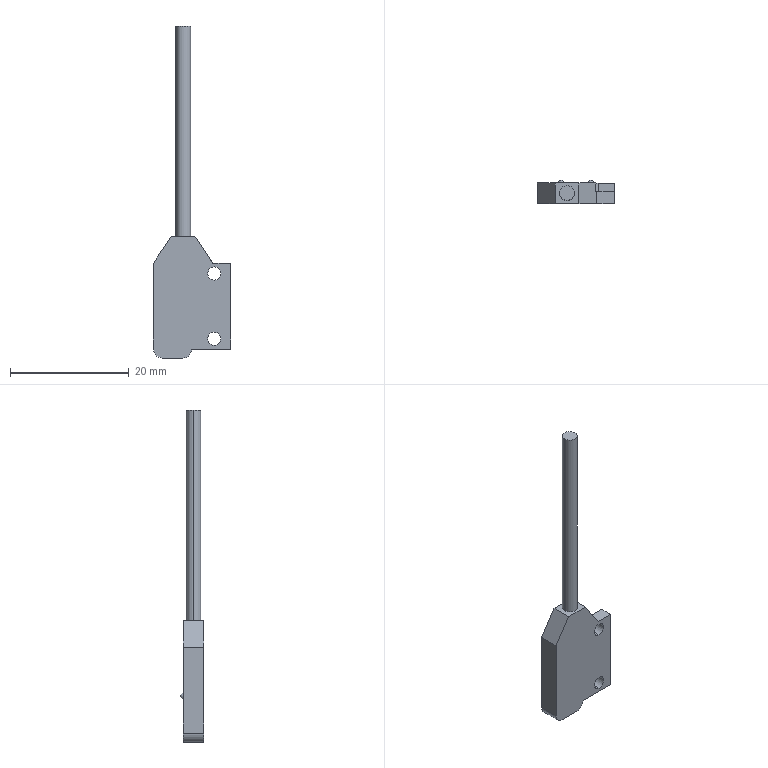Part | SolidWorks | features ICE 4, Chamfer 2, Fillet 2, Extrusion 1 | 1 solid | 28 faces | box 13 x 4 x 56 mm | volume 912.44 mm3 | plane 16 | cylinder 10 | sphere 2 | commonest cylinder face diameters 2.2 x4 2.5 x2 3 x2 4 x2
STEP:
#1=CARTESIAN_POINT('',(-0.25,1.75,47.25));
#2=VERTEX_POINT('',#1);
#3=CARTESIAN_POINT('',(-2.75,1.75,47.25));
#4=VERTEX_POINT('',#3);
#5=CARTESIAN_POINT('',(-1.5,1.75,47.25));
#6=DIRECTION('',(0.,0.,1.));
#7=DIRECTION('',(1.,0.,0.));
#8=AXIS2_PLACEMENT_3D('',#5,#6,#7);
#9=CIRCLE('',#8,1.25);
#10=EDGE_CURVE('',#2,#4,#9,.T.);
#11=ORIENTED_EDGE('',*,*,#10,.F.);
#12=CARTESIAN_POINT('',(-0.25,1.75,11.75));
#13=VERTEX_POINT('',#12);
#14=CARTESIAN_POINT('',(-0.25,1.75,47.25));
#15=DIRECTION('',(0.,0.,-1.));
#16=VECTOR('',#15,1000.);
#17=LINE('',#14,#16);
#18=EDGE_CURVE('',#2,#13,#17,.T.);
#19=ORIENTED_EDGE('',*,*,#18,.T.);
#20=CARTESIAN_POINT('',(-2.75,1.75,11.75));
#21=VERTEX_POINT('',#20);
#22=CARTESIAN_POINT('',(-1.5,1.75,11.75));
#23=DIRECTION('',(0.,0.,1.));
#24=DIRECTION('',(-1.,0.,0.));
#25=AXIS2_PLACEMENT_3D('',#22,#23,#24);
#26=CIRCLE('',#25,1.25);
#27=EDGE_CURVE('',#13,#21,#26,.T.);
#28=ORIENTED_EDGE('',*,*,#27,.T.);
#29=CARTESIAN_POINT('',(-2.75,1.75,47.25));
#30=DIRECTION('',(0.,0.,-1.));
#31=VECTOR('',#30,1000.);
#32=LINE('',#29,#31);
#33=EDGE_CURVE('',#4,#21,#32,.T.);
#34=ORIENTED_EDGE('',*,*,#33,.F.);
#35=EDGE_LOOP('',(#11,#19,#28,#34));
#36=FACE_OUTER_BOUND('',#35,.T.);
#37=CARTESIAN_POINT('',(-1.5,1.75,47.25));
#38=DIRECTION('',(0.,0.,-1.));
#39=DIRECTION('',(-1.,0.,0.));
#40=AXIS2_PLACEMENT_3D('',#37,#38,#39);
#41=CYLINDRICAL_SURFACE('',#40,1.25);
#42=ADVANCED_FACE('',(#36),#41,.T.);
#43=CARTESIAN_POINT('',(3.75,0.,-6.6));
#44=VERTEX_POINT('',#43);
#45=CARTESIAN_POINT('',(3.75,0.,-4.4));
#46=VERTEX_POINT('',#45);
#47=CARTESIAN_POINT('',(3.75,0.,-5.5));
#48=DIRECTION('',(0.,1.,0.));
#49=DIRECTION('',(0.,0.,1.));
#50=AXIS2_PLACEMENT_3D('',#47,#48,#49);
#51=CIRCLE('',#50,1.1);
#52=EDGE_CURVE('',#44,#46,#51,.T.);
#53=ORIENTED_EDGE('',*,*,#52,.F.);
#54=CARTESIAN_POINT('',(3.75,2.1,-6.6));
#55=VERTEX_POINT('',#54);
#56=CARTESIAN_POINT('',(3.75,-1.5,-6.6));
#57=DIRECTION('',(0.,1.,0.));
#58=VECTOR('',#57,1000.);
#59=LINE('',#56,#58);
#60=EDGE_CURVE('',#44,#55,#59,.T.);
#61=ORIENTED_EDGE('',*,*,#60,.T.);
#62=CARTESIAN_POINT('',(3.75,2.1,-4.4));
#63=VERTEX_POINT('',#62);
#64=CARTESIAN_POINT('',(3.75,2.1,-5.5));
#65=DIRECTION('',(0.,-1.,0.));
#66=DIRECTION('',(0.,0.,1.));
#67=AXIS2_PLACEMENT_3D('',#64,#65,#66);
#68=CIRCLE('',#67,1.1);
#69=EDGE_CURVE('',#63,#55,#68,.T.);
#70=ORIENTED_EDGE('',*,*,#69,.F.);
#71=CARTESIAN_POINT('',(3.75,-1.5,-4.4));
#72=DIRECTION('',(0.,1.,0.));
#73=VECTOR('',#72,1000.);
#74=LINE('',#71,#73);
#75=EDGE_CURVE('',#46,#63,#74,.T.);
#76=ORIENTED_EDGE('',*,*,#75,.F.);
#77=EDGE_LOOP('',(#53,#61,#70,#76));
#78=FACE_OUTER_BOUND('',#77,.T.);
#79=CARTESIAN_POINT('',(3.75,-1.5,-5.5));
#80=DIRECTION('',(0.,1.,0.));
#81=DIRECTION('',(0.,0.,1.));
#82=AXIS2_PLACEMENT_3D('',#79,#80,#81);
#83=CYLINDRICAL_SURFACE('',#82,1.1);
#84=ADVANCED_FACE('',(#78),#83,.F.);
#85=CARTESIAN_POINT('',(3.75,0.,4.4));
#86=VERTEX_POINT('',#85);
#87=CARTESIAN_POINT('',(3.75,0.,6.6));
#88=VERTEX_POINT('',#87);
#89=CARTESIAN_POINT('',(3.75,0.,5.5));
#90=DIRECTION('',(0.,1.,0.));
#91=DIRECTION('',(0.,0.,1.));
#92=AXIS2_PLACEMENT_3D('',#89,#90,#91);
#93=CIRCLE('',#92,1.1);
#94=EDGE_CURVE('',#86,#88,#93,.T.);
#95=ORIENTED_EDGE('',*,*,#94,.F.);
#96=CARTESIAN_POINT('',(3.75,2.1,4.4));
#97=VERTEX_POINT('',#96);
#98=CARTESIAN_POINT('',(3.75,-1.5,4.4));
#99=DIRECTION('',(0.,1.,0.));
#100=VECTOR('',#99,1000.);
#101=LINE('',#98,#100);
#102=EDGE_CURVE('',#86,#97,#101,.T.);
#103=ORIENTED_EDGE('',*,*,#102,.T.);
#104=CARTESIAN_POINT('',(3.75,2.1,6.6));
#105=VERTEX_POINT('',#104);
#106=CARTESIAN_POINT('',(3.75,2.1,5.5));
#107=DIRECTION('',(0.,-1.,0.));
#108=DIRECTION('',(0.,0.,1.));
#109=AXIS2_PLACEMENT_3D('',#106,#107,#108);
#110=CIRCLE('',#109,1.1);
#111=EDGE_CURVE('',#105,#97,#110,.T.);
#112=ORIENTED_EDGE('',*,*,#111,.F.);
#113=CARTESIAN_POINT('',(3.75,-1.5,6.6));
#114=DIRECTION('',(0.,1.,0.));
#115=VECTOR('',#114,1000.);
#116=LINE('',#113,#115);
#117=EDGE_CURVE('',#88,#105,#116,.T.);
#118=ORIENTED_EDGE('',*,*,#117,.F.);
#119=EDGE_LOOP('',(#95,#103,#112,#118));
#120=FACE_OUTER_BOUND('',#119,.T.);
#121=CARTESIAN_POINT('',(3.75,-1.5,5.5));
#122=DIRECTION('',(0.,1.,0.));
#123=DIRECTION('',(0.,0.,1.));
#124=AXIS2_PLACEMENT_3D('',#121,#122,#123);
#125=CYLINDRICAL_SURFACE('',#124,1.1);
#126=ADVANCED_FACE('',(#120),#125,.F.);
#127=CARTESIAN_POINT('',(3.5,2.1,7.25));
#128=VERTEX_POINT('',#127);
#129=CARTESIAN_POINT('',(6.5,2.1,7.25));
#130=VERTEX_POINT('',#129);
#131=CARTESIAN_POINT('',(3.5,2.1,7.25));
#132=DIRECTION('',(1.,0.,0.));
#133=VECTOR('',#132,1000.);
#134=LINE('',#131,#133);
#135=EDGE_CURVE('',#128,#130,#134,.T.);
#136=ORIENTED_EDGE('',*,*,#135,.F.);
#137=CARTESIAN_POINT('',(3.5,0.,7.25));
#138=VERTEX_POINT('',#137);
#139=CARTESIAN_POINT('',(3.5,3.5,7.25));
#140=DIRECTION('',(0.,-1.,0.));
#141=VECTOR('',#140,1000.);
#142=LINE('',#139,#141);
#143=EDGE_CURVE('',#128,#138,#142,.T.);
#144=ORIENTED_EDGE('',*,*,#143,.T.);
#145=CARTESIAN_POINT('',(6.5,0.,7.25));
#146=VERTEX_POINT('',#145);
#147=CARTESIAN_POINT('',(3.5,0.,7.25));
#148=DIRECTION('',(1.,0.,0.));
#149=VECTOR('',#148,1000.);
#150=LINE('',#147,#149);
#151=EDGE_CURVE('',#138,#146,#150,.T.);
#152=ORIENTED_EDGE('',*,*,#151,.T.);
#153=CARTESIAN_POINT('',(6.5,3.5,7.25));
#154=DIRECTION('',(0.,-1.,0.));
#155=VECTOR('',#154,1000.);
#156=LINE('',#153,#155);
#157=EDGE_CURVE('',#130,#146,#156,.T.);
#158=ORIENTED_EDGE('',*,*,#157,.F.);
#159=EDGE_LOOP('',(#136,#144,#152,#158));
#160=FACE_OUTER_BOUND('',#159,.T.);
#161=CARTESIAN_POINT('',(3.5,3.5,7.25));
#162=DIRECTION('',(0.,0.,-1.));
#163=DIRECTION('',(-1.,0.,0.));
#164=AXIS2_PLACEMENT_3D('',#161,#162,#163);
#165=PLANE('',#164);
#166=ADVANCED_FACE('',(#160),#165,.F.);
#167=ORIENTED_EDGE('',*,*,#102,.F.);
#168=CARTESIAN_POINT('',(3.75,0.,5.5));
#169=DIRECTION('',(0.,1.,0.));
#170=DIRECTION('',(0.,0.,1.));
#171=AXIS2_PLACEMENT_3D('',#168,#169,#170);
#172=CIRCLE('',#171,1.1);
#173=EDGE_CURVE('',#88,#86,#172,.T.);
#174=ORIENTED_EDGE('',*,*,#173,.F.);
#175=ORIENTED_EDGE('',*,*,#117,.T.);
#176=CARTESIAN_POINT('',(3.75,2.1,5.5));
#177=DIRECTION('',(0.,-1.,0.));
#178=DIRECTION('',(0.,0.,1.));
#179=AXIS2_PLACEMENT_3D('',#176,#177,#178);
#180=CIRCLE('',#179,1.1);
#181=EDGE_CURVE('',#97,#105,#180,.T.);
#182=ORIENTED_EDGE('',*,*,#181,.F.);
#183=EDGE_LOOP('',(#167,#174,#175,#182));
#184=FACE_OUTER_BOUND('',#183,.T.);
#185=CARTESIAN_POINT('',(3.75,-1.5,5.5));
#186=DIRECTION('',(0.,1.,0.));
#187=DIRECTION('',(0.,0.,1.));
#188=AXIS2_PLACEMENT_3D('',#185,#186,#187);
#189=CYLINDRICAL_SURFACE('',#188,1.1);
#190=ADVANCED_FACE('',(#184),#189,.F.);
#191=ORIENTED_EDGE('',*,*,#60,.F.);
#192=CARTESIAN_POINT('',(3.75,0.,-5.5));
#193=DIRECTION('',(0.,1.,0.));
#194=DIRECTION('',(0.,0.,1.));
#195=AXIS2_PLACEMENT_3D('',#192,#193,#194);
#196=CIRCLE('',#195,1.1);
#197=EDGE_CURVE('',#46,#44,#196,.T.);
#198=ORIENTED_EDGE('',*,*,#197,.F.);
#199=ORIENTED_EDGE('',*,*,#75,.T.);
#200=CARTESIAN_POINT('',(3.75,2.1,-5.5));
#201=DIRECTION('',(0.,-1.,0.));
#202=DIRECTION('',(0.,0.,1.));
#203=AXIS2_PLACEMENT_3D('',#200,#201,#202);
#204=CIRCLE('',#203,1.1);
#205=EDGE_CURVE('',#55,#63,#204,.T.);
#206=ORIENTED_EDGE('',*,*,#205,.F.);
#207=EDGE_LOOP('',(#191,#198,#199,#206));
#208=FACE_OUTER_BOUND('',#207,.T.);
#209=CARTESIAN_POINT('',(3.75,-1.5,-5.5));
#210=DIRECTION('',(0.,1.,0.));
#211=DIRECTION('',(0.,0.,1.));
#212=AXIS2_PLACEMENT_3D('',#209,#210,#211);
#213=CYLINDRICAL_SURFACE('',#212,1.1);
#214=ADVANCED_FACE('',(#208),#213,.F.);
#215=CARTESIAN_POINT('',(3.75,3.5,3.5));
#216=VERTEX_POINT('',#215);
#217=CARTESIAN_POINT('',(3.359,3.5,7.461));
#218=VERTEX_POINT('',#217);
#219=CARTESIAN_POINT('',(3.75,3.5,5.5));
#220=DIRECTION('',(0.,1.,0.));
#221=DIRECTION('',(0.,0.,1.));
#222=AXIS2_PLACEMENT_3D('',#219,#220,#221);
#223=CIRCLE('',#222,2.);
#224=EDGE_CURVE('',#216,#218,#223,.T.);
#225=ORIENTED_EDGE('',*,*,#224,.F.);
#226=CARTESIAN_POINT('',(6.5,3.5,3.5));
#227=VERTEX_POINT('',#226);
#228=CARTESIAN_POINT('',(3.75,3.5,3.5));
#229=DIRECTION('',(-1.,0.,0.));
#230=VECTOR('',#229,1000.);
#231=LINE('',#228,#230);
#232=EDGE_CURVE('',#227,#216,#231,.T.);
#233=ORIENTED_EDGE('',*,*,#232,.F.);
#234=CARTESIAN_POINT('',(6.5,3.5,-3.5));
#235=VERTEX_POINT('',#234);
#236=CARTESIAN_POINT('',(6.5,3.5,-7.25));
#237=DIRECTION('',(0.,0.,-1.));
#238=VECTOR('',#237,1000.);
#239=LINE('',#236,#238);
#240=EDGE_CURVE('',#227,#235,#239,.T.);
#241=ORIENTED_EDGE('',*,*,#240,.T.);
#242=CARTESIAN_POINT('',(3.75,3.5,-3.5));
#243=VERTEX_POINT('',#242);
#244=CARTESIAN_POINT('',(3.75,3.5,-3.5));
#245=DIRECTION('',(1.,0.,0.));
#246=VECTOR('',#245,1000.);
#247=LINE('',#244,#246);
#248=EDGE_CURVE('',#243,#235,#247,.T.);
#249=ORIENTED_EDGE('',*,*,#248,.F.);
#250=CARTESIAN_POINT('',(1.75,3.5,-5.5));
#251=VERTEX_POINT('',#250);
#252=CARTESIAN_POINT('',(3.75,3.5,-5.5));
#253=DIRECTION('',(0.,1.,0.));
#254=DIRECTION('',(0.,0.,1.));
#255=AXIS2_PLACEMENT_3D('',#252,#253,#254);
#256=CIRCLE('',#255,2.);
#257=EDGE_CURVE('',#251,#243,#256,.T.);
#258=ORIENTED_EDGE('',*,*,#257,.F.);
#259=CARTESIAN_POINT('',(1.75,3.5,-7.25));
#260=VERTEX_POINT('',#259);
#261=CARTESIAN_POINT('',(1.75,3.5,-7.25));
#262=DIRECTION('',(0.,0.,1.));
#263=VECTOR('',#262,1000.);
#264=LINE('',#261,#263);
#265=EDGE_CURVE('',#260,#251,#264,.T.);
#266=ORIENTED_EDGE('',*,*,#265,.F.);
#267=CARTESIAN_POINT('',(-0.05,3.5,-7.25));
#268=VERTEX_POINT('',#267);
#269=CARTESIAN_POINT('',(-0.05,3.5,-7.25));
#270=DIRECTION('',(-1.,0.,0.));
#271=VECTOR('',#270,1000.);
#272=LINE('',#269,#271);
#273=EDGE_CURVE('',#260,#268,#272,.T.);
#274=ORIENTED_EDGE('',*,*,#273,.T.);
#275=CARTESIAN_POINT('',(-1.55,3.5,-8.75));
#276=VERTEX_POINT('',#275);
#277=CARTESIAN_POINT('',(-1.55,3.5,-7.25));
#278=DIRECTION('',(0.,1.,0.));
#279=DIRECTION('',(0.,0.,1.));
#280=AXIS2_PLACEMENT_3D('',#277,#278,#279);
#281=CIRCLE('',#280,1.5);
#282=EDGE_CURVE('',#268,#276,#281,.T.);
#283=ORIENTED_EDGE('',*,*,#282,.T.);
#284=CARTESIAN_POINT('',(-5.,3.5,-8.75));
#285=VERTEX_POINT('',#284);
#286=CARTESIAN_POINT('',(-6.5,3.5,-8.75));
#287=DIRECTION('',(-1.,0.,0.));
#288=VECTOR('',#287,1000.);
#289=LINE('',#286,#288);
#290=EDGE_CURVE('',#276,#285,#289,.T.);
#291=ORIENTED_EDGE('',*,*,#290,.T.);
#292=CARTESIAN_POINT('',(-6.5,3.5,-7.25));
#293=VERTEX_POINT('',#292);
#294=CARTESIAN_POINT('',(-5.,3.5,-7.25));
#295=DIRECTION('',(0.,1.,0.));
#296=DIRECTION('',(0.,0.,1.));
#297=AXIS2_PLACEMENT_3D('',#294,#295,#296);
#298=CIRCLE('',#297,1.5);
#299=EDGE_CURVE('',#285,#293,#298,.T.);
#300=ORIENTED_EDGE('',*,*,#299,.T.);
#301=CARTESIAN_POINT('',(-6.5,3.5,7.25));
#302=VERTEX_POINT('',#301);
#303=CARTESIAN_POINT('',(-6.5,3.5,-8.75));
#304=DIRECTION('',(0.,0.,1.));
#305=VECTOR('',#304,1000.);
#306=LINE('',#303,#305);
#307=EDGE_CURVE('',#293,#302,#306,.T.);
#308=ORIENTED_EDGE('',*,*,#307,.T.);
#309=CARTESIAN_POINT('',(-3.5,3.5,11.75));
#310=VERTEX_POINT('',#309);
#311=CARTESIAN_POINT('',(-7.846,3.5,5.231));
#312=DIRECTION('',(0.5547,0.,0.8321));
#313=VECTOR('',#312,1000.);
#314=LINE('',#311,#313);
#315=EDGE_CURVE('',#302,#310,#314,.T.);
#316=ORIENTED_EDGE('',*,*,#315,.T.);
#317=CARTESIAN_POINT('',(0.5,3.5,11.75));
#318=VERTEX_POINT('',#317);
#319=CARTESIAN_POINT('',(-6.5,3.5,11.75));
#320=DIRECTION('',(1.,0.,0.));
#321=VECTOR('',#320,1000.);
#322=LINE('',#319,#321);
#323=EDGE_CURVE('',#310,#318,#322,.T.);
#324=ORIENTED_EDGE('',*,*,#323,.T.);
#325=CARTESIAN_POINT('',(5.769,3.5,3.846));
#326=DIRECTION('',(0.5547,0.,-0.8321));
#327=VECTOR('',#326,1000.);
#328=LINE('',#325,#327);
#329=EDGE_CURVE('',#318,#218,#328,.T.);
#330=ORIENTED_EDGE('',*,*,#329,.T.);
#331=EDGE_LOOP('',(#225,#233,#241,#249,#258,#266,#274,#283,#291,#300,#308,#316,#324,#330));
#332=FACE_OUTER_BOUND('',#331,.T.);
#333=CARTESIAN_POINT('',(-2.5,3.5,-0.5));
#334=VERTEX_POINT('',#333);
#335=CARTESIAN_POINT('',(-2.5,3.5,-1.5));
#336=VERTEX_POINT('',#335);
#337=CARTESIAN_POINT('',(-2.5,3.5,-1.));
#338=DIRECTION('',(0.,1.,0.));
#339=DIRECTION('',(0.,0.,1.));
#340=AXIS2_PLACEMENT_3D('',#337,#338,#339);
#341=CIRCLE('',#340,0.5);
#342=EDGE_CURVE('',#334,#336,#341,.T.);
#343=ORIENTED_EDGE('',*,*,#342,.F.);
#344=CARTESIAN_POINT('',(-2.5,3.5,-1.));
#345=DIRECTION('',(0.,1.,0.));
#346=DIRECTION('',(0.,0.,1.));
#347=AXIS2_PLACEMENT_3D('',#344,#345,#346);
#348=CIRCLE('',#347,0.5);
#349=EDGE_CURVE('',#336,#334,#348,.T.);
#350=ORIENTED_EDGE('',*,*,#349,.F.);
#351=EDGE_LOOP('',(#343,#350));
#352=FACE_BOUND('',#351,.T.);
#353=CARTESIAN_POINT('',(2.5,3.5,-1.5));
#354=VERTEX_POINT('',#353);
#355=CARTESIAN_POINT('',(2.5,3.5,-0.5));
#356=VERTEX_POINT('',#355);
#357=CARTESIAN_POINT('',(2.5,3.5,-1.));
#358=DIRECTION('',(0.,1.,0.));
#359=DIRECTION('',(0.,0.,-1.));
#360=AXIS2_PLACEMENT_3D('',#357,#358,#359);
#361=CIRCLE('',#360,0.5);
#362=EDGE_CURVE('',#354,#356,#361,.T.);
#363=ORIENTED_EDGE('',*,*,#362,.F.);
#364=CARTESIAN_POINT('',(2.5,3.5,-1.));
#365=DIRECTION('',(0.,1.,0.));
#366=DIRECTION('',(0.,0.,-1.));
#367=AXIS2_PLACEMENT_3D('',#364,#365,#366);
#368=CIRCLE('',#367,0.5);
#369=EDGE_CURVE('',#356,#354,#368,.T.);
#370=ORIENTED_EDGE('',*,*,#369,.F.);
#371=EDGE_LOOP('',(#363,#370));
#372=FACE_BOUND('',#371,.T.);
#373=CARTESIAN_POINT('',(0.,3.5,0.));
#374=DIRECTION('',(0.,1.,0.));
#375=DIRECTION('',(0.,0.,1.));
#376=AXIS2_PLACEMENT_3D('',#373,#374,#375);
#377=PLANE('',#376);
#378=ADVANCED_FACE('',(#332,#352,#372),#377,.T.);
#379=CARTESIAN_POINT('',(-3.5,0.,11.75));
#380=VERTEX_POINT('',#379);
#381=CARTESIAN_POINT('',(0.5,0.,11.75));
#382=VERTEX_POINT('',#381);
#383=CARTESIAN_POINT('',(-6.5,0.,11.75));
#384=DIRECTION('',(1.,0.,0.));
#385=VECTOR('',#384,1000.);
#386=LINE('',#383,#385);
#387=EDGE_CURVE('',#380,#382,#386,.T.);
#388=ORIENTED_EDGE('',*,*,#387,.T.);
#389=CARTESIAN_POINT('',(0.5,3.5,11.75));
#390=DIRECTION('',(0.,1.,0.));
#391=VECTOR('',#390,1000.);
#392=LINE('',#389,#391);
#393=EDGE_CURVE('',#382,#318,#392,.T.);
#394=ORIENTED_EDGE('',*,*,#393,.T.);
#395=ORIENTED_EDGE('',*,*,#323,.F.);
#396=CARTESIAN_POINT('',(-3.5,3.5,11.75));
#397=DIRECTION('',(0.,-1.,0.));
#398=VECTOR('',#397,1000.);
#399=LINE('',#396,#398);
#400=EDGE_CURVE('',#310,#380,#399,.T.);
#401=ORIENTED_EDGE('',*,*,#400,.T.);
#402=EDGE_LOOP('',(#388,#394,#395,#401));
#403=FACE_OUTER_BOUND('',#402,.T.);
#404=CARTESIAN_POINT('',(-1.5,1.75,11.75));
#405=DIRECTION('',(0.,0.,1.));
#406=DIRECTION('',(-1.,0.,0.));
#407=AXIS2_PLACEMENT_3D('',#404,#405,#406);
#408=CIRCLE('',#407,1.25);
#409=EDGE_CURVE('',#21,#13,#408,.T.);
#410=ORIENTED_EDGE('',*,*,#409,.F.);
#411=ORIENTED_EDGE('',*,*,#27,.F.);
#412=EDGE_LOOP('',(#410,#411));
#413=FACE_BOUND('',#412,.T.);
#414=CARTESIAN_POINT('',(-6.5,3.5,11.75));
#415=DIRECTION('',(0.,0.,-1.));
#416=DIRECTION('',(-1.,0.,0.));
#417=AXIS2_PLACEMENT_3D('',#414,#415,#416);
#418=PLANE('',#417);
#419=ADVANCED_FACE('',(#403,#413),#418,.F.);
#420=ORIENTED_EDGE('',*,*,#240,.F.);
#421=CARTESIAN_POINT('',(6.5,2.1,3.5));
#422=VERTEX_POINT('',#421);
#423=CARTESIAN_POINT('',(6.5,2.1,3.5));
#424=DIRECTION('',(0.,1.,0.));
#425=VECTOR('',#424,1000.);
#426=LINE('',#423,#425);
#427=EDGE_CURVE('',#422,#227,#426,.T.);
#428=ORIENTED_EDGE('',*,*,#427,.F.);
#429=CARTESIAN_POINT('',(6.5,2.1,3.5));
#430=DIRECTION('',(0.,0.,-1.));
#431=VECTOR('',#430,1000.);
#432=LINE('',#429,#431);
#433=EDGE_CURVE('',#130,#422,#432,.T.);
#434=ORIENTED_EDGE('',*,*,#433,.F.);
#435=ORIENTED_EDGE('',*,*,#157,.T.);
#436=CARTESIAN_POINT('',(6.5,0.,-7.25));
#437=VERTEX_POINT('',#436);
#438=CARTESIAN_POINT('',(6.5,0.,-7.25));
#439=DIRECTION('',(0.,0.,-1.));
#440=VECTOR('',#439,1000.);
#441=LINE('',#438,#440);
#442=EDGE_CURVE('',#146,#437,#441,.T.);
#443=ORIENTED_EDGE('',*,*,#442,.T.);
#444=CARTESIAN_POINT('',(6.5,2.1,-7.25));
#445=VERTEX_POINT('',#444);
#446=CARTESIAN_POINT('',(6.5,3.5,-7.25));
#447=DIRECTION('',(0.,-1.,0.));
#448=VECTOR('',#447,1000.);
#449=LINE('',#446,#448);
#450=EDGE_CURVE('',#445,#437,#449,.T.);
#451=ORIENTED_EDGE('',*,*,#450,.F.);
#452=CARTESIAN_POINT('',(6.5,2.1,-3.5));
#453=VERTEX_POINT('',#452);
#454=CARTESIAN_POINT('',(6.5,2.1,-7.25));
#455=DIRECTION('',(0.,0.,-1.));
#456=VECTOR('',#455,1000.);
#457=LINE('',#454,#456);
#458=EDGE_CURVE('',#453,#445,#457,.T.);
#459=ORIENTED_EDGE('',*,*,#458,.F.);
#460=CARTESIAN_POINT('',(6.5,2.1,-3.5));
#461=DIRECTION('',(0.,1.,0.));
#462=VECTOR('',#461,1000.);
#463=LINE('',#460,#462);
#464=EDGE_CURVE('',#453,#235,#463,.T.);
#465=ORIENTED_EDGE('',*,*,#464,.T.);
#466=EDGE_LOOP('',(#420,#428,#434,#435,#443,#451,#459,#465));
#467=FACE_OUTER_BOUND('',#466,.T.);
#468=CARTESIAN_POINT('',(6.5,3.5,-7.25));
#469=DIRECTION('',(-1.,0.,0.));
#470=DIRECTION('',(0.,0.,1.));
#471=AXIS2_PLACEMENT_3D('',#468,#469,#470);
#472=PLANE('',#471);
#473=ADVANCED_FACE('',(#467),#472,.F.);
#474=ORIENTED_EDGE('',*,*,#273,.F.);
#475=CARTESIAN_POINT('',(1.75,2.1,-7.25));
#476=VERTEX_POINT('',#475);
#477=CARTESIAN_POINT('',(1.75,2.1,-7.25));
#478=DIRECTION('',(0.,1.,0.));
#479=VECTOR('',#478,1000.);
#480=LINE('',#477,#479);
#481=EDGE_CURVE('',#476,#260,#480,.T.);
#482=ORIENTED_EDGE('',*,*,#481,.F.);
#483=CARTESIAN_POINT('',(6.5,2.1,-7.25));
#484=DIRECTION('',(-1.,0.,0.));
#485=VECTOR('',#484,1000.);
#486=LINE('',#483,#485);
#487=EDGE_CURVE('',#445,#476,#486,.T.);
#488=ORIENTED_EDGE('',*,*,#487,.F.);
#489=ORIENTED_EDGE('',*,*,#450,.T.);
#490=CARTESIAN_POINT('',(-0.05,0.,-7.25));
#491=VERTEX_POINT('',#490);
#492=CARTESIAN_POINT('',(-0.05,0.,-7.25));
#493=DIRECTION('',(-1.,0.,0.));
#494=VECTOR('',#493,1000.);
#495=LINE('',#492,#494);
#496=EDGE_CURVE('',#437,#491,#495,.T.);
#497=ORIENTED_EDGE('',*,*,#496,.T.);
#498=CARTESIAN_POINT('',(-0.05,3.5,-7.25));
#499=DIRECTION('',(0.,-1.,0.));
#500=VECTOR('',#499,1000.);
#501=LINE('',#498,#500);
#502=EDGE_CURVE('',#268,#491,#501,.T.);
#503=ORIENTED_EDGE('',*,*,#502,.F.);
#504=EDGE_LOOP('',(#474,#482,#488,#489,#497,#503));
#505=FACE_OUTER_BOUND('',#504,.T.);
#506=CARTESIAN_POINT('',(-0.05,3.5,-7.25));
#507=DIRECTION('',(0.,0.,1.));
#508=DIRECTION('',(1.,0.,0.));
#509=AXIS2_PLACEMENT_3D('',#506,#507,#508);
#510=PLANE('',#509);
#511=ADVANCED_FACE('',(#505),#510,.F.);
#512=ORIENTED_EDGE('',*,*,#290,.F.);
#513=CARTESIAN_POINT('',(-1.55,0.,-8.75));
#514=VERTEX_POINT('',#513);
#515=CARTESIAN_POINT('',(-1.55,3.5,-8.75));
#516=DIRECTION('',(0.,-1.,0.));
#517=VECTOR('',#516,1000.);
#518=LINE('',#515,#517);
#519=EDGE_CURVE('',#276,#514,#518,.T.);
#520=ORIENTED_EDGE('',*,*,#519,.T.);
#521=CARTESIAN_POINT('',(-5.,0.,-8.75));
#522=VERTEX_POINT('',#521);
#523=CARTESIAN_POINT('',(-6.5,0.,-8.75));
#524=DIRECTION('',(-1.,0.,0.));
#525=VECTOR('',#524,1000.);
#526=LINE('',#523,#525);
#527=EDGE_CURVE('',#514,#522,#526,.T.);
#528=ORIENTED_EDGE('',*,*,#527,.T.);
#529=CARTESIAN_POINT('',(-5.,3.5,-8.75));
#530=DIRECTION('',(0.,1.,0.));
#531=VECTOR('',#530,1000.);
#532=LINE('',#529,#531);
#533=EDGE_CURVE('',#522,#285,#532,.T.);
#534=ORIENTED_EDGE('',*,*,#533,.T.);
#535=EDGE_LOOP('',(#512,#520,#528,#534));
#536=FACE_OUTER_BOUND('',#535,.T.);
#537=CARTESIAN_POINT('',(-6.5,3.5,-8.75));
#538=DIRECTION('',(0.,0.,1.));
#539=DIRECTION('',(1.,0.,0.));
#540=AXIS2_PLACEMENT_3D('',#537,#538,#539);
#541=PLANE('',#540);
#542=ADVANCED_FACE('',(#536),#541,.F.);
#543=ORIENTED_EDGE('',*,*,#307,.F.);
#544=CARTESIAN_POINT('',(-6.5,0.,-7.25));
#545=VERTEX_POINT('',#544);
#546=CARTESIAN_POINT('',(-6.5,3.5,-7.25));
#547=DIRECTION('',(0.,-1.,0.));
#548=VECTOR('',#547,1000.);
#549=LINE('',#546,#548);
#550=EDGE_CURVE('',#293,#545,#549,.T.);
#551=ORIENTED_EDGE('',*,*,#550,.T.);
#552=CARTESIAN_POINT('',(-6.5,0.,7.25));
#553=VERTEX_POINT('',#552);
#554=CARTESIAN_POINT('',(-6.5,0.,-8.75));
#555=DIRECTION('',(0.,0.,1.));
#556=VECTOR('',#555,1000.);
#557=LINE('',#554,#556);
#558=EDGE_CURVE('',#545,#553,#557,.T.);
#559=ORIENTED_EDGE('',*,*,#558,.T.);
#560=CARTESIAN_POINT('',(-6.5,3.5,7.25));
#561=DIRECTION('',(0.,1.,0.));
#562=VECTOR('',#561,1000.);
#563=LINE('',#560,#562);
#564=EDGE_CURVE('',#553,#302,#563,.T.);
#565=ORIENTED_EDGE('',*,*,#564,.T.);
#566=EDGE_LOOP('',(#543,#551,#559,#565));
#567=FACE_OUTER_BOUND('',#566,.T.);
#568=CARTESIAN_POINT('',(-6.5,3.5,-8.75));
#569=DIRECTION('',(1.,0.,0.));
#570=DIRECTION('',(0.,0.,-1.));
#571=AXIS2_PLACEMENT_3D('',#568,#569,#570);
#572=PLANE('',#571);
#573=ADVANCED_FACE('',(#567),#572,.F.);
#574=ORIENTED_EDGE('',*,*,#173,.T.);
#575=ORIENTED_EDGE('',*,*,#94,.T.);
#576=EDGE_LOOP('',(#574,#575));
#577=FACE_BOUND('',#576,.T.);
#578=ORIENTED_EDGE('',*,*,#197,.T.);
#579=ORIENTED_EDGE('',*,*,#52,.T.);
#580=EDGE_LOOP('',(#578,#579));
#581=FACE_BOUND('',#580,.T.);
#582=ORIENTED_EDGE('',*,*,#527,.F.);
#583=CARTESIAN_POINT('',(-1.55,0.,-7.25));
#584=DIRECTION('',(0.,-1.,0.));
#585=DIRECTION('',(0.,0.,1.));
#586=AXIS2_PLACEMENT_3D('',#583,#584,#585);
#587=CIRCLE('',#586,1.5);
#588=EDGE_CURVE('',#514,#491,#587,.T.);
#589=ORIENTED_EDGE('',*,*,#588,.T.);
#590=ORIENTED_EDGE('',*,*,#496,.F.);
#591=ORIENTED_EDGE('',*,*,#442,.F.);
#592=ORIENTED_EDGE('',*,*,#151,.F.);
#593=CARTESIAN_POINT('',(3.5,0.,7.25));
#594=DIRECTION('',(-0.5547,0.,0.8321));
#595=VECTOR('',#594,1000.);
#596=LINE('',#593,#595);
#597=EDGE_CURVE('',#138,#382,#596,.T.);
#598=ORIENTED_EDGE('',*,*,#597,.T.);
#599=ORIENTED_EDGE('',*,*,#387,.F.);
#600=CARTESIAN_POINT('',(-3.5,0.,11.75));
#601=DIRECTION('',(-0.5547,0.,-0.8321));
#602=VECTOR('',#601,1000.);
#603=LINE('',#600,#602);
#604=EDGE_CURVE('',#380,#553,#603,.T.);
#605=ORIENTED_EDGE('',*,*,#604,.T.);
#606=ORIENTED_EDGE('',*,*,#558,.F.);
#607=CARTESIAN_POINT('',(-5.,0.,-7.25));
#608=DIRECTION('',(0.,-1.,0.));
#609=DIRECTION('',(0.,0.,1.));
#610=AXIS2_PLACEMENT_3D('',#607,#608,#609);
#611=CIRCLE('',#610,1.5);
#612=EDGE_CURVE('',#545,#522,#611,.T.);
#613=ORIENTED_EDGE('',*,*,#612,.T.);
#614=EDGE_LOOP('',(#582,#589,#590,#591,#592,#598,#599,#605,#606,#613));
#615=FACE_OUTER_BOUND('',#614,.T.);
#616=CARTESIAN_POINT('',(0.,0.,0.));
#617=DIRECTION('',(0.,1.,0.));
#618=DIRECTION('',(0.,0.,1.));
#619=AXIS2_PLACEMENT_3D('',#616,#617,#618);
#620=PLANE('',#619);
#621=ADVANCED_FACE('',(#577,#581,#615),#620,.F.);
#622=ORIENTED_EDGE('',*,*,#315,.F.);
#623=ORIENTED_EDGE('',*,*,#564,.F.);
#624=ORIENTED_EDGE('',*,*,#604,.F.);
#625=ORIENTED_EDGE('',*,*,#400,.F.);
#626=EDGE_LOOP('',(#622,#623,#624,#625));
#627=FACE_OUTER_BOUND('',#626,.T.);
#628=CARTESIAN_POINT('',(-3.5,3.5,11.75));
#629=DIRECTION('',(0.8321,0.,-0.5547));
#630=DIRECTION('',(0.,-1.,0.));
#631=AXIS2_PLACEMENT_3D('',#628,#629,#630);
#632=PLANE('',#631);
#633=ADVANCED_FACE('',(#627),#632,.F.);
#634=CARTESIAN_POINT('',(3.359,2.1,7.461));
#635=VERTEX_POINT('',#634);
#636=CARTESIAN_POINT('',(3.359,2.1,7.461));
#637=DIRECTION('',(0.,-1.,0.));
#638=VECTOR('',#637,1000.);
#639=LINE('',#636,#638);
#640=EDGE_CURVE('',#218,#635,#639,.T.);
#641=ORIENTED_EDGE('',*,*,#640,.F.);
#642=ORIENTED_EDGE('',*,*,#329,.F.);
#643=ORIENTED_EDGE('',*,*,#393,.F.);
#644=ORIENTED_EDGE('',*,*,#597,.F.);
#645=ORIENTED_EDGE('',*,*,#143,.F.);
#646=CARTESIAN_POINT('',(3.5,2.1,7.25));
#647=DIRECTION('',(-0.5547,0.,0.8321));
#648=VECTOR('',#647,1000.);
#649=LINE('',#646,#648);
#650=EDGE_CURVE('',#128,#635,#649,.T.);
#651=ORIENTED_EDGE('',*,*,#650,.T.);
#652=EDGE_LOOP('',(#641,#642,#643,#644,#645,#651));
#653=FACE_OUTER_BOUND('',#652,.T.);
#654=CARTESIAN_POINT('',(3.5,3.5,7.25));
#655=DIRECTION('',(-0.8321,0.,-0.5547));
#656=DIRECTION('',(0.,-1.,0.));
#657=AXIS2_PLACEMENT_3D('',#654,#655,#656);
#658=PLANE('',#657);
#659=ADVANCED_FACE('',(#653),#658,.F.);
#660=ORIENTED_EDGE('',*,*,#18,.F.);
#661=CARTESIAN_POINT('',(-1.5,1.75,47.25));
#662=DIRECTION('',(0.,0.,1.));
#663=DIRECTION('',(1.,0.,0.));
#664=AXIS2_PLACEMENT_3D('',#661,#662,#663);
#665=CIRCLE('',#664,1.25);
#666=EDGE_CURVE('',#4,#2,#665,.T.);
#667=ORIENTED_EDGE('',*,*,#666,.F.);
#668=ORIENTED_EDGE('',*,*,#33,.T.);
#669=ORIENTED_EDGE('',*,*,#409,.T.);
#670=EDGE_LOOP('',(#660,#667,#668,#669));
#671=FACE_OUTER_BOUND('',#670,.T.);
#672=CARTESIAN_POINT('',(-1.5,1.75,47.25));
#673=DIRECTION('',(0.,0.,-1.));
#674=DIRECTION('',(-1.,0.,0.));
#675=AXIS2_PLACEMENT_3D('',#672,#673,#674);
#676=CYLINDRICAL_SURFACE('',#675,1.25);
#677=ADVANCED_FACE('',(#671),#676,.T.);
#678=ORIENTED_EDGE('',*,*,#666,.T.);
#679=ORIENTED_EDGE('',*,*,#10,.T.);
#680=EDGE_LOOP('',(#678,#679));
#681=FACE_OUTER_BOUND('',#680,.T.);
#682=CARTESIAN_POINT('',(-1.5,1.75,47.25));
#683=DIRECTION('',(0.,0.,1.));
#684=DIRECTION('',(1.,0.,0.));
#685=AXIS2_PLACEMENT_3D('',#682,#683,#684);
#686=PLANE('',#685);
#687=ADVANCED_FACE('',(#681),#686,.T.);
#688=ORIENTED_EDGE('',*,*,#282,.F.);
#689=ORIENTED_EDGE('',*,*,#502,.T.);
#690=ORIENTED_EDGE('',*,*,#588,.F.);
#691=ORIENTED_EDGE('',*,*,#519,.F.);
#692=EDGE_LOOP('',(#688,#689,#690,#691));
#693=FACE_OUTER_BOUND('',#692,.T.);
#694=CARTESIAN_POINT('',(-1.55,3.5,-7.25));
#695=DIRECTION('',(0.,-1.,0.));
#696=DIRECTION('',(0.,0.,-1.));
#697=AXIS2_PLACEMENT_3D('',#694,#695,#696);
#698=CYLINDRICAL_SURFACE('',#697,1.5);
#699=ADVANCED_FACE('',(#693),#698,.T.);
#700=ORIENTED_EDGE('',*,*,#299,.F.);
#701=ORIENTED_EDGE('',*,*,#533,.F.);
#702=ORIENTED_EDGE('',*,*,#612,.F.);
#703=ORIENTED_EDGE('',*,*,#550,.F.);
#704=EDGE_LOOP('',(#700,#701,#702,#703));
#705=FACE_OUTER_BOUND('',#704,.T.);
#706=CARTESIAN_POINT('',(-5.,3.5,-7.25));
#707=DIRECTION('',(0.,-1.,0.));
#708=DIRECTION('',(0.,0.,-1.));
#709=AXIS2_PLACEMENT_3D('',#706,#707,#708);
#710=CYLINDRICAL_SURFACE('',#709,1.5);
#711=ADVANCED_FACE('',(#705),#710,.T.);
#712=ORIENTED_EDGE('',*,*,#362,.T.);
#713=ORIENTED_EDGE('',*,*,#369,.T.);
#714=EDGE_LOOP('',(#712,#713));
#715=FACE_OUTER_BOUND('',#714,.T.);
#716=CARTESIAN_POINT('',(2.5,3.5,-1.));
#717=DIRECTION('',(0.,1.,0.));
#718=DIRECTION('',(1.,0.,0.));
#719=AXIS2_PLACEMENT_3D('',#716,#717,#718);
#720=SPHERICAL_SURFACE('',#719,0.5);
#721=ADVANCED_FACE('',(#715),#720,.T.);
#722=ORIENTED_EDGE('',*,*,#342,.T.);
#723=ORIENTED_EDGE('',*,*,#349,.T.);
#724=EDGE_LOOP('',(#722,#723));
#725=FACE_OUTER_BOUND('',#724,.T.);
#726=CARTESIAN_POINT('',(-2.5,3.5,-1.));
#727=DIRECTION('',(0.,1.,0.));
#728=DIRECTION('',(1.,0.,0.));
#729=AXIS2_PLACEMENT_3D('',#726,#727,#728);
#730=SPHERICAL_SURFACE('',#729,0.5);
#731=ADVANCED_FACE('',(#725),#730,.T.);
#732=ORIENTED_EDGE('',*,*,#458,.T.);
#733=ORIENTED_EDGE('',*,*,#487,.T.);
#734=CARTESIAN_POINT('',(1.75,2.1,-5.5));
#735=VERTEX_POINT('',#734);
#736=CARTESIAN_POINT('',(1.75,2.1,-7.25));
#737=DIRECTION('',(0.,0.,1.));
#738=VECTOR('',#737,1000.);
#739=LINE('',#736,#738);
#740=EDGE_CURVE('',#476,#735,#739,.T.);
#741=ORIENTED_EDGE('',*,*,#740,.T.);
#742=CARTESIAN_POINT('',(3.75,2.1,-3.5));
#743=VERTEX_POINT('',#742);
#744=CARTESIAN_POINT('',(3.75,2.1,-5.5));
#745=DIRECTION('',(0.,1.,0.));
#746=DIRECTION('',(0.,0.,1.));
#747=AXIS2_PLACEMENT_3D('',#744,#745,#746);
#748=CIRCLE('',#747,2.);
#749=EDGE_CURVE('',#735,#743,#748,.T.);
#750=ORIENTED_EDGE('',*,*,#749,.T.);
#751=CARTESIAN_POINT('',(3.75,2.1,-3.5));
#752=DIRECTION('',(1.,0.,0.));
#753=VECTOR('',#752,1000.);
#754=LINE('',#751,#753);
#755=EDGE_CURVE('',#743,#453,#754,.T.);
#756=ORIENTED_EDGE('',*,*,#755,.T.);
#757=EDGE_LOOP('',(#732,#733,#741,#750,#756));
#758=FACE_OUTER_BOUND('',#757,.T.);
#759=ORIENTED_EDGE('',*,*,#69,.T.);
#760=ORIENTED_EDGE('',*,*,#205,.T.);
#761=EDGE_LOOP('',(#759,#760));
#762=FACE_BOUND('',#761,.T.);
#763=CARTESIAN_POINT('',(3.75,2.1,-5.5));
#764=DIRECTION('',(0.,1.,0.));
#765=DIRECTION('',(0.,0.,1.));
#766=AXIS2_PLACEMENT_3D('',#763,#764,#765);
#767=PLANE('',#766);
#768=ADVANCED_FACE('',(#758,#762),#767,.T.);
#769=ORIENTED_EDGE('',*,*,#248,.T.);
#770=ORIENTED_EDGE('',*,*,#464,.F.);
#771=ORIENTED_EDGE('',*,*,#755,.F.);
#772=CARTESIAN_POINT('',(3.75,2.1,-3.5));
#773=DIRECTION('',(0.,1.,0.));
#774=VECTOR('',#773,1000.);
#775=LINE('',#772,#774);
#776=EDGE_CURVE('',#743,#243,#775,.T.);
#777=ORIENTED_EDGE('',*,*,#776,.T.);
#778=EDGE_LOOP('',(#769,#770,#771,#777));
#779=FACE_OUTER_BOUND('',#778,.T.);
#780=CARTESIAN_POINT('',(3.75,2.1,-3.5));
#781=DIRECTION('',(0.,0.,1.));
#782=DIRECTION('',(1.,0.,0.));
#783=AXIS2_PLACEMENT_3D('',#780,#781,#782);
#784=PLANE('',#783);
#785=ADVANCED_FACE('',(#779),#784,.F.);
#786=ORIENTED_EDGE('',*,*,#257,.T.);
#787=ORIENTED_EDGE('',*,*,#776,.F.);
#788=ORIENTED_EDGE('',*,*,#749,.F.);
#789=CARTESIAN_POINT('',(1.75,2.1,-5.5));
#790=DIRECTION('',(0.,1.,0.));
#791=VECTOR('',#790,1000.);
#792=LINE('',#789,#791);
#793=EDGE_CURVE('',#735,#251,#792,.T.);
#794=ORIENTED_EDGE('',*,*,#793,.T.);
#795=EDGE_LOOP('',(#786,#787,#788,#794));
#796=FACE_OUTER_BOUND('',#795,.T.);
#797=CARTESIAN_POINT('',(3.75,2.1,-5.5));
#798=DIRECTION('',(0.,1.,0.));
#799=DIRECTION('',(0.,0.,1.));
#800=AXIS2_PLACEMENT_3D('',#797,#798,#799);
#801=CYLINDRICAL_SURFACE('',#800,2.);
#802=ADVANCED_FACE('',(#796),#801,.F.);
#803=ORIENTED_EDGE('',*,*,#265,.T.);
#804=ORIENTED_EDGE('',*,*,#793,.F.);
#805=ORIENTED_EDGE('',*,*,#740,.F.);
#806=ORIENTED_EDGE('',*,*,#481,.T.);
#807=EDGE_LOOP('',(#803,#804,#805,#806));
#808=FACE_OUTER_BOUND('',#807,.T.);
#809=CARTESIAN_POINT('',(1.75,2.1,-7.25));
#810=DIRECTION('',(-1.,0.,0.));
#811=DIRECTION('',(0.,0.,1.));
#812=AXIS2_PLACEMENT_3D('',#809,#810,#811);
#813=PLANE('',#812);
#814=ADVANCED_FACE('',(#808),#813,.F.);
#815=ORIENTED_EDGE('',*,*,#111,.T.);
#816=ORIENTED_EDGE('',*,*,#181,.T.);
#817=EDGE_LOOP('',(#815,#816));
#818=FACE_BOUND('',#817,.T.);
#819=ORIENTED_EDGE('',*,*,#135,.T.);
#820=ORIENTED_EDGE('',*,*,#433,.T.);
#821=CARTESIAN_POINT('',(3.75,2.1,3.5));
#822=VERTEX_POINT('',#821);
#823=CARTESIAN_POINT('',(3.75,2.1,3.5));
#824=DIRECTION('',(-1.,0.,0.));
#825=VECTOR('',#824,1000.);
#826=LINE('',#823,#825);
#827=EDGE_CURVE('',#422,#822,#826,.T.);
#828=ORIENTED_EDGE('',*,*,#827,.T.);
#829=CARTESIAN_POINT('',(3.75,2.1,5.5));
#830=DIRECTION('',(0.,1.,0.));
#831=DIRECTION('',(0.,0.,1.));
#832=AXIS2_PLACEMENT_3D('',#829,#830,#831);
#833=CIRCLE('',#832,2.);
#834=EDGE_CURVE('',#822,#635,#833,.T.);
#835=ORIENTED_EDGE('',*,*,#834,.T.);
#836=ORIENTED_EDGE('',*,*,#650,.F.);
#837=EDGE_LOOP('',(#819,#820,#828,#835,#836));
#838=FACE_OUTER_BOUND('',#837,.T.);
#839=CARTESIAN_POINT('',(3.75,2.1,5.5));
#840=DIRECTION('',(0.,1.,0.));
#841=DIRECTION('',(0.,0.,1.));
#842=AXIS2_PLACEMENT_3D('',#839,#840,#841);
#843=PLANE('',#842);
#844=ADVANCED_FACE('',(#818,#838),#843,.T.);
#845=ORIENTED_EDGE('',*,*,#640,.T.);
#846=ORIENTED_EDGE('',*,*,#834,.F.);
#847=CARTESIAN_POINT('',(3.75,2.1,3.5));
#848=DIRECTION('',(0.,1.,0.));
#849=VECTOR('',#848,1000.);
#850=LINE('',#847,#849);
#851=EDGE_CURVE('',#822,#216,#850,.T.);
#852=ORIENTED_EDGE('',*,*,#851,.T.);
#853=ORIENTED_EDGE('',*,*,#224,.T.);
#854=EDGE_LOOP('',(#845,#846,#852,#853));
#855=FACE_OUTER_BOUND('',#854,.T.);
#856=CARTESIAN_POINT('',(3.75,2.1,5.5));
#857=DIRECTION('',(0.,1.,0.));
#858=DIRECTION('',(0.,0.,1.));
#859=AXIS2_PLACEMENT_3D('',#856,#857,#858);
#860=CYLINDRICAL_SURFACE('',#859,2.);
#861=ADVANCED_FACE('',(#855),#860,.F.);
#862=ORIENTED_EDGE('',*,*,#232,.T.);
#863=ORIENTED_EDGE('',*,*,#851,.F.);
#864=ORIENTED_EDGE('',*,*,#827,.F.);
#865=ORIENTED_EDGE('',*,*,#427,.T.);
#866=EDGE_LOOP('',(#862,#863,#864,#865));
#867=FACE_OUTER_BOUND('',#866,.T.);
#868=CARTESIAN_POINT('',(3.75,2.1,3.5));
#869=DIRECTION('',(0.,0.,-1.));
#870=DIRECTION('',(-1.,0.,0.));
#871=AXIS2_PLACEMENT_3D('',#868,#869,#870);
#872=PLANE('',#871);
#873=ADVANCED_FACE('',(#867),#872,.F.);
#874=CLOSED_SHELL('',(#42,#84,#126,#166,#190,#214,#378,#419,#473,#511,#542,#573,#621,#633,#659,#677,#687,#699,#711,#721,#731,#768,#785,#802,#814,#844,#861,#873));
#875=MANIFOLD_SOLID_BREP('',#874);
#876=CARTESIAN_POINT('',(0.,0.,0.));
#877=DIRECTION('',(0.,0.,1.));
#878=DIRECTION('',(1.,0.,0.));
#879=AXIS2_PLACEMENT_3D('',#876,#877,#878);
#880=(LENGTH_UNIT()NAMED_UNIT(*)SI_UNIT(.MILLI.,.METRE.));
#881=UNCERTAINTY_MEASURE_WITH_UNIT(LENGTH_MEASURE(0.00001),#880,'','');
#882=(NAMED_UNIT(*)PLANE_ANGLE_UNIT()SI_UNIT($,.RADIAN.));
#883=(NAMED_UNIT(*)SI_UNIT($,.STERADIAN.)SOLID_ANGLE_UNIT());
#884=(GEOMETRIC_REPRESENTATION_CONTEXT(3)GLOBAL_UNCERTAINTY_ASSIGNED_CONTEXT((#881))GLOBAL_UNIT_ASSIGNED_CONTEXT((#880,#882,#883))REPRESENTATION_CONTEXT('',''));
#885=ADVANCED_BREP_SHAPE_REPRESENTATION('',(#875,#879),#884);